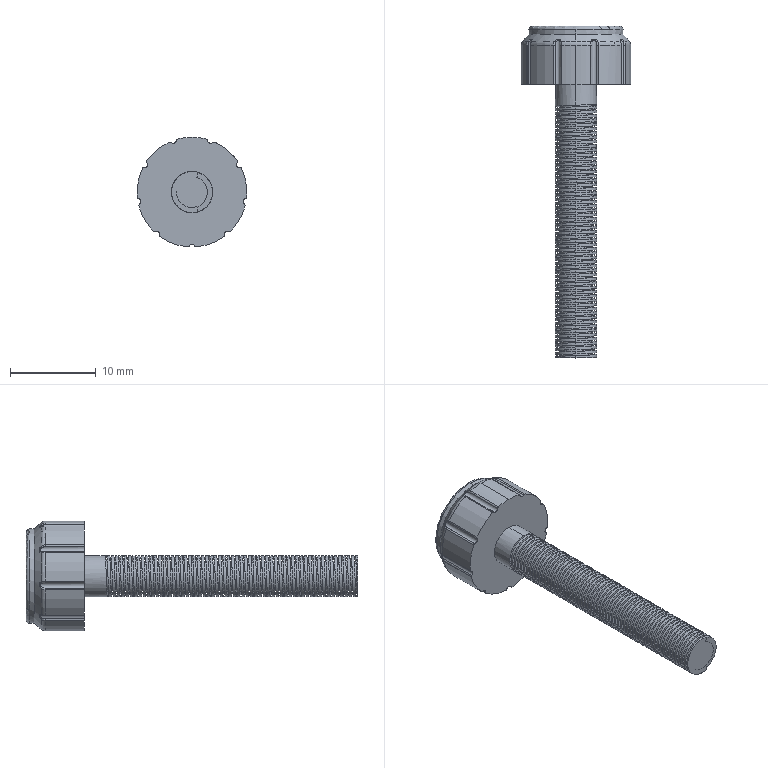Part | SolidWorks | features BaseBody 1 | 1 solid | 257 faces | box 12.8 x 38.7 x 12.78 mm | volume 1300 mm3 | cylinder 166 | spline 73 | torus 12 | plane 4 | cone 2 | commonest cylinder face diameters 4.8 x120 0.4 x22 0.692 x12 12.8 x10 11 x2